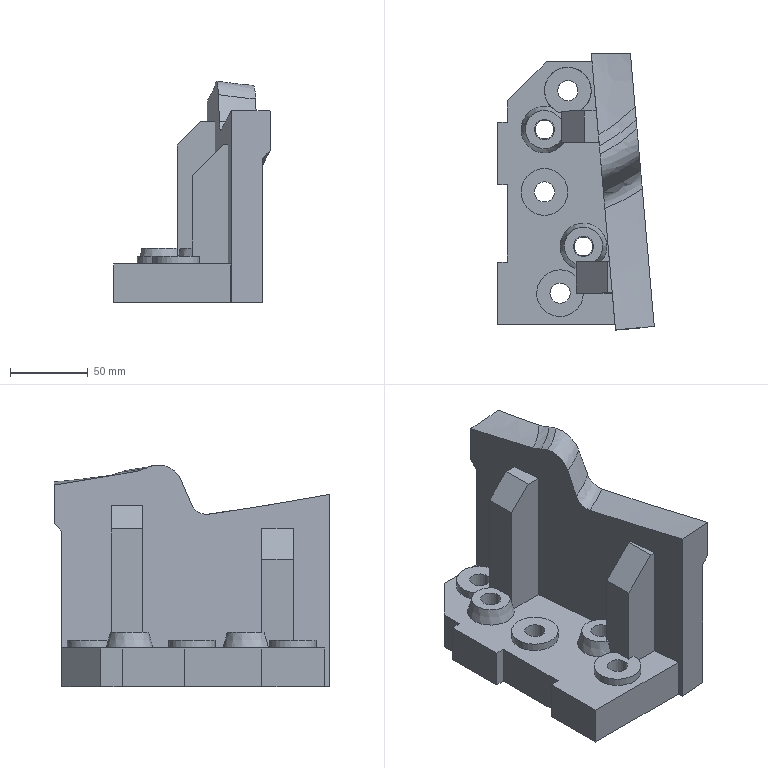Part | NX | features solid 2 | 1 solid | 56 faces | box 100.469 x 177.111 x 142.435 mm | volume 798040 mm3 | plane 36 | cylinder 10 | spline 8 | cone 2 | commonest cylinder face diameters 13 x5 30 x3 12 x2